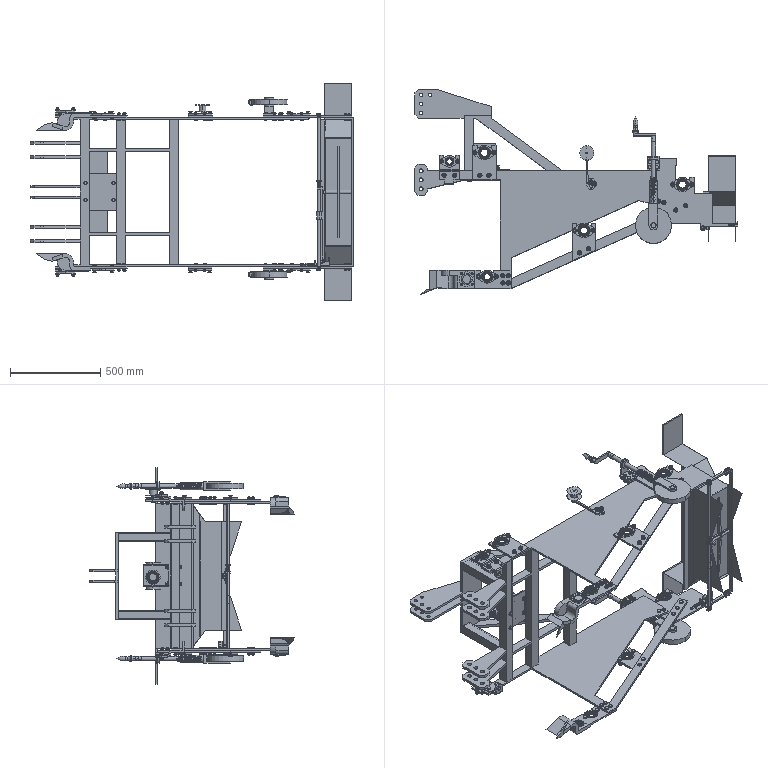Part | SolidWorks | features CompositeCurve 9, InContextFeatHolder 1 | 269 solids | 11920 faces | volume 26128597 mm3 | cone 5110 | plane 2793 | cylinder 2022 | sphere 1200 | torus 762 | spline 33 | commonest cylinder face diameters 12 x454 6 x256 10 x164 25 x147 13 x120 18 x112